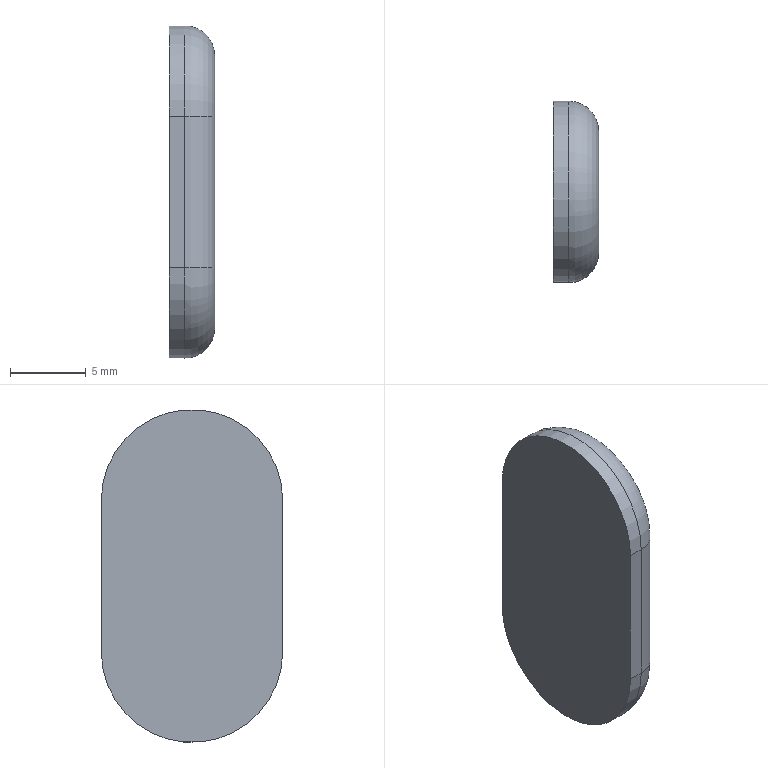Part | STEP file | 1-26.4 | 1 solid | 10 faces | box 3 x 12 x 22 mm | volume 652.172 mm3 | plane 4 | cylinder 4 | torus 2 | commonest cylinder face diameters 4 x2 12 x2
STEP:
#1=CARTESIAN_POINT('',(0.,0.,0.));
#2=DIRECTION('',(0.,0.,1.));
#3=DIRECTION('',(1.,0.,0.));
#4=AXIS2_PLACEMENT_3D('',#1,#2,#3);
#5=CARTESIAN_POINT('',(-3.,6.,5.));
#6=VERTEX_POINT('',#5);
#7=CARTESIAN_POINT('',(-3.,-6.,5.));
#8=VERTEX_POINT('',#7);
#9=CARTESIAN_POINT('',(-3.,0.,5.));
#10=DIRECTION('',(1.,0.,0.));
#11=DIRECTION('',(0.,1.,0.));
#12=AXIS2_PLACEMENT_3D('',#9,#10,#11);
#13=CIRCLE('',#12,6.);
#14=CARTESIAN_POINT('',(-3.,5.,0.));
#15=DIRECTION('',(1.,0.,0.));
#16=DIRECTION('',(0.,1.,0.));
#17=AXIS2_PLACEMENT_3D('',#14,#15,#16);
#18=PLANE('',#17);
#19=CARTESIAN_POINT('',(-5.,5.));
#20=DIRECTION('',(1.,0.));
#21=AXIS2_PLACEMENT_2D('',#19,#20);
#22=CIRCLE('',#21,6.);
#23=(GEOMETRIC_REPRESENTATION_CONTEXT(2)PARAMETRIC_REPRESENTATION_CONTEXT()REPRESENTATION_CONTEXT('',''));
#24=DEFINITIONAL_REPRESENTATION('',(#22),#23);
#25=PCURVE('',#18,#24);
#26=CARTESIAN_POINT('',(0.,0.,5.));
#27=DIRECTION('',(-1.,0.,0.));
#28=DIRECTION('',(0.,1.,0.));
#29=AXIS2_PLACEMENT_3D('',#26,#27,#28);
#30=CYLINDRICAL_SURFACE('',#29,6.);
#31=CARTESIAN_POINT('',(6.283,3.));
#32=DIRECTION('',(-1.,0.));
#33=VECTOR('',#32,1.);
#34=LINE('',#31,#33);
#35=(GEOMETRIC_REPRESENTATION_CONTEXT(2)PARAMETRIC_REPRESENTATION_CONTEXT()REPRESENTATION_CONTEXT('',''));
#36=DEFINITIONAL_REPRESENTATION('',(#34),#35);
#37=PCURVE('',#30,#36);
#38=SURFACE_CURVE('',#13,(#25,#37),.PCURVE_S1.);
#39=EDGE_CURVE('',#6,#8,#38,.T.);
#40=ORIENTED_EDGE('',*,*,#39,.T.);
#41=CARTESIAN_POINT('',(-3.,-6.,-5.));
#42=VERTEX_POINT('',#41);
#43=CARTESIAN_POINT('',(-3.,-6.,5.));
#44=DIRECTION('',(0.,0.,-1.));
#45=VECTOR('',#44,1.);
#46=LINE('',#43,#45);
#47=CARTESIAN_POINT('',(-11.,5.));
#48=DIRECTION('',(0.,-1.));
#49=VECTOR('',#48,1.);
#50=LINE('',#47,#49);
#51=(GEOMETRIC_REPRESENTATION_CONTEXT(2)PARAMETRIC_REPRESENTATION_CONTEXT()REPRESENTATION_CONTEXT('',''));
#52=DEFINITIONAL_REPRESENTATION('',(#50),#51);
#53=PCURVE('',#18,#52);
#54=CARTESIAN_POINT('',(-1.5,-6.,0.));
#55=DIRECTION('',(0.,1.,0.));
#56=DIRECTION('',(0.,0.,-1.));
#57=AXIS2_PLACEMENT_3D('',#54,#55,#56);
#58=PLANE('',#57);
#59=CARTESIAN_POINT('',(-5.,1.5));
#60=DIRECTION('',(1.,0.));
#61=VECTOR('',#60,1.);
#62=LINE('',#59,#61);
#63=(GEOMETRIC_REPRESENTATION_CONTEXT(2)PARAMETRIC_REPRESENTATION_CONTEXT()REPRESENTATION_CONTEXT('',''));
#64=DEFINITIONAL_REPRESENTATION('',(#62),#63);
#65=PCURVE('',#58,#64);
#66=SURFACE_CURVE('',#46,(#53,#65),.PCURVE_S1.);
#67=EDGE_CURVE('',#8,#42,#66,.T.);
#68=ORIENTED_EDGE('',*,*,#67,.T.);
#69=CARTESIAN_POINT('',(-3.,6.,-5.));
#70=VERTEX_POINT('',#69);
#71=CARTESIAN_POINT('',(-3.,0.,-5.));
#72=DIRECTION('',(1.,0.,0.));
#73=DIRECTION('',(0.,-1.,0.));
#74=AXIS2_PLACEMENT_3D('',#71,#72,#73);
#75=CIRCLE('',#74,6.);
#76=CARTESIAN_POINT('',(-5.,-5.));
#77=DIRECTION('',(-1.,0.));
#78=AXIS2_PLACEMENT_2D('',#76,#77);
#79=CIRCLE('',#78,6.);
#80=(GEOMETRIC_REPRESENTATION_CONTEXT(2)PARAMETRIC_REPRESENTATION_CONTEXT()REPRESENTATION_CONTEXT('',''));
#81=DEFINITIONAL_REPRESENTATION('',(#79),#80);
#82=PCURVE('',#18,#81);
#83=CARTESIAN_POINT('',(0.,0.,-5.));
#84=DIRECTION('',(-1.,0.,0.));
#85=DIRECTION('',(0.,-1.,0.));
#86=AXIS2_PLACEMENT_3D('',#83,#84,#85);
#87=CYLINDRICAL_SURFACE('',#86,6.);
#88=CARTESIAN_POINT('',(6.283,3.));
#89=DIRECTION('',(-1.,0.));
#90=VECTOR('',#89,1.);
#91=LINE('',#88,#90);
#92=(GEOMETRIC_REPRESENTATION_CONTEXT(2)PARAMETRIC_REPRESENTATION_CONTEXT()REPRESENTATION_CONTEXT('',''));
#93=DEFINITIONAL_REPRESENTATION('',(#91),#92);
#94=PCURVE('',#87,#93);
#95=SURFACE_CURVE('',#75,(#82,#94),.PCURVE_S1.);
#96=EDGE_CURVE('',#42,#70,#95,.T.);
#97=ORIENTED_EDGE('',*,*,#96,.T.);
#98=CARTESIAN_POINT('',(-3.,6.,-5.));
#99=DIRECTION('',(0.,0.,1.));
#100=VECTOR('',#99,1.);
#101=LINE('',#98,#100);
#102=CARTESIAN_POINT('',(1.,-5.));
#103=DIRECTION('',(0.,1.));
#104=VECTOR('',#103,1.);
#105=LINE('',#102,#104);
#106=(GEOMETRIC_REPRESENTATION_CONTEXT(2)PARAMETRIC_REPRESENTATION_CONTEXT()REPRESENTATION_CONTEXT('',''));
#107=DEFINITIONAL_REPRESENTATION('',(#105),#106);
#108=PCURVE('',#18,#107);
#109=CARTESIAN_POINT('',(-1.5,6.,0.));
#110=DIRECTION('',(0.,-1.,0.));
#111=DIRECTION('',(0.,0.,1.));
#112=AXIS2_PLACEMENT_3D('',#109,#110,#111);
#113=PLANE('',#112);
#114=CARTESIAN_POINT('',(-5.,1.5));
#115=DIRECTION('',(1.,0.));
#116=VECTOR('',#115,1.);
#117=LINE('',#114,#116);
#118=(GEOMETRIC_REPRESENTATION_CONTEXT(2)PARAMETRIC_REPRESENTATION_CONTEXT()REPRESENTATION_CONTEXT('',''));
#119=DEFINITIONAL_REPRESENTATION('',(#117),#118);
#120=PCURVE('',#113,#119);
#121=SURFACE_CURVE('',#101,(#108,#120),.PCURVE_S1.);
#122=EDGE_CURVE('',#70,#6,#121,.T.);
#123=ORIENTED_EDGE('',*,*,#122,.T.);
#124=EDGE_LOOP('',(#40,#68,#97,#123));
#125=FACE_BOUND('',#124,.F.);
#126=ADVANCED_FACE('',(#125),#18,.F.);
#127=CARTESIAN_POINT('',(0.,4.,5.));
#128=VERTEX_POINT('',#127);
#129=CARTESIAN_POINT('',(0.,-4.,5.));
#130=VERTEX_POINT('',#129);
#131=CARTESIAN_POINT('',(0.,0.,5.));
#132=DIRECTION('',(1.,0.,0.));
#133=DIRECTION('',(0.,1.,0.));
#134=AXIS2_PLACEMENT_3D('',#131,#132,#133);
#135=CIRCLE('',#134,4.);
#136=CARTESIAN_POINT('',(0.,5.,0.));
#137=DIRECTION('',(1.,0.,0.));
#138=DIRECTION('',(0.,1.,0.));
#139=AXIS2_PLACEMENT_3D('',#136,#137,#138);
#140=PLANE('',#139);
#141=CARTESIAN_POINT('',(-5.,5.));
#142=DIRECTION('',(1.,0.));
#143=AXIS2_PLACEMENT_2D('',#141,#142);
#144=CIRCLE('',#143,4.);
#145=(GEOMETRIC_REPRESENTATION_CONTEXT(2)PARAMETRIC_REPRESENTATION_CONTEXT()REPRESENTATION_CONTEXT('',''));
#146=DEFINITIONAL_REPRESENTATION('',(#144),#145);
#147=PCURVE('',#140,#146);
#148=CARTESIAN_POINT('',(-2.,0.,5.));
#149=DIRECTION('',(-1.,0.,0.));
#150=DIRECTION('',(0.,1.,0.));
#151=AXIS2_PLACEMENT_3D('',#148,#149,#150);
#152=TOROIDAL_SURFACE('',#151,4.,2.);
#153=CARTESIAN_POINT('',(6.283,4.712));
#154=DIRECTION('',(-1.,0.));
#155=VECTOR('',#154,1.);
#156=LINE('',#153,#155);
#157=(GEOMETRIC_REPRESENTATION_CONTEXT(2)PARAMETRIC_REPRESENTATION_CONTEXT()REPRESENTATION_CONTEXT('',''));
#158=DEFINITIONAL_REPRESENTATION('',(#156),#157);
#159=PCURVE('',#152,#158);
#160=SURFACE_CURVE('',#135,(#147,#159),.PCURVE_S1.);
#161=EDGE_CURVE('',#128,#130,#160,.T.);
#162=ORIENTED_EDGE('',*,*,#161,.T.);
#163=CARTESIAN_POINT('',(0.,-4.,-5.));
#164=VERTEX_POINT('',#163);
#165=CARTESIAN_POINT('',(0.,-4.,5.));
#166=DIRECTION('',(0.,0.,-1.));
#167=VECTOR('',#166,1.);
#168=LINE('',#165,#167);
#169=CARTESIAN_POINT('',(-9.,5.));
#170=DIRECTION('',(0.,-1.));
#171=VECTOR('',#170,1.);
#172=LINE('',#169,#171);
#173=(GEOMETRIC_REPRESENTATION_CONTEXT(2)PARAMETRIC_REPRESENTATION_CONTEXT()REPRESENTATION_CONTEXT('',''));
#174=DEFINITIONAL_REPRESENTATION('',(#172),#173);
#175=PCURVE('',#140,#174);
#176=CARTESIAN_POINT('',(-2.,-4.,5.));
#177=DIRECTION('',(0.,0.,-1.));
#178=DIRECTION('',(1.,0.,0.));
#179=AXIS2_PLACEMENT_3D('',#176,#177,#178);
#180=CYLINDRICAL_SURFACE('',#179,2.);
#181=CARTESIAN_POINT('',(0.,0.));
#182=DIRECTION('',(0.,1.));
#183=VECTOR('',#182,1.);
#184=LINE('',#181,#183);
#185=(GEOMETRIC_REPRESENTATION_CONTEXT(2)PARAMETRIC_REPRESENTATION_CONTEXT()REPRESENTATION_CONTEXT('',''));
#186=DEFINITIONAL_REPRESENTATION('',(#184),#185);
#187=PCURVE('',#180,#186);
#188=SURFACE_CURVE('',#168,(#175,#187),.PCURVE_S1.);
#189=EDGE_CURVE('',#130,#164,#188,.T.);
#190=ORIENTED_EDGE('',*,*,#189,.T.);
#191=CARTESIAN_POINT('',(0.,4.,-5.));
#192=VERTEX_POINT('',#191);
#193=CARTESIAN_POINT('',(0.,0.,-5.));
#194=DIRECTION('',(1.,0.,0.));
#195=DIRECTION('',(0.,-1.,0.));
#196=AXIS2_PLACEMENT_3D('',#193,#194,#195);
#197=CIRCLE('',#196,4.);
#198=CARTESIAN_POINT('',(-5.,-5.));
#199=DIRECTION('',(-1.,0.));
#200=AXIS2_PLACEMENT_2D('',#198,#199);
#201=CIRCLE('',#200,4.);
#202=(GEOMETRIC_REPRESENTATION_CONTEXT(2)PARAMETRIC_REPRESENTATION_CONTEXT()REPRESENTATION_CONTEXT('',''));
#203=DEFINITIONAL_REPRESENTATION('',(#201),#202);
#204=PCURVE('',#140,#203);
#205=CARTESIAN_POINT('',(-2.,0.,-5.));
#206=DIRECTION('',(-1.,0.,0.));
#207=DIRECTION('',(0.,-1.,0.));
#208=AXIS2_PLACEMENT_3D('',#205,#206,#207);
#209=TOROIDAL_SURFACE('',#208,4.,2.);
#210=CARTESIAN_POINT('',(6.283,4.712));
#211=DIRECTION('',(-1.,0.));
#212=VECTOR('',#211,1.);
#213=LINE('',#210,#212);
#214=(GEOMETRIC_REPRESENTATION_CONTEXT(2)PARAMETRIC_REPRESENTATION_CONTEXT()REPRESENTATION_CONTEXT('',''));
#215=DEFINITIONAL_REPRESENTATION('',(#213),#214);
#216=PCURVE('',#209,#215);
#217=SURFACE_CURVE('',#197,(#204,#216),.PCURVE_S1.);
#218=EDGE_CURVE('',#164,#192,#217,.T.);
#219=ORIENTED_EDGE('',*,*,#218,.T.);
#220=CARTESIAN_POINT('',(0.,4.,-5.));
#221=DIRECTION('',(0.,0.,1.));
#222=VECTOR('',#221,1.);
#223=LINE('',#220,#222);
#224=CARTESIAN_POINT('',(-1.,-5.));
#225=DIRECTION('',(0.,1.));
#226=VECTOR('',#225,1.);
#227=LINE('',#224,#226);
#228=(GEOMETRIC_REPRESENTATION_CONTEXT(2)PARAMETRIC_REPRESENTATION_CONTEXT()REPRESENTATION_CONTEXT('',''));
#229=DEFINITIONAL_REPRESENTATION('',(#227),#228);
#230=PCURVE('',#140,#229);
#231=CARTESIAN_POINT('',(-2.,4.,-5.));
#232=DIRECTION('',(0.,0.,1.));
#233=DIRECTION('',(1.,0.,0.));
#234=AXIS2_PLACEMENT_3D('',#231,#232,#233);
#235=CYLINDRICAL_SURFACE('',#234,2.);
#236=CARTESIAN_POINT('',(0.,0.));
#237=DIRECTION('',(0.,1.));
#238=VECTOR('',#237,1.);
#239=LINE('',#236,#238);
#240=(GEOMETRIC_REPRESENTATION_CONTEXT(2)PARAMETRIC_REPRESENTATION_CONTEXT()REPRESENTATION_CONTEXT('',''));
#241=DEFINITIONAL_REPRESENTATION('',(#239),#240);
#242=PCURVE('',#235,#241);
#243=SURFACE_CURVE('',#223,(#230,#242),.PCURVE_S1.);
#244=EDGE_CURVE('',#192,#128,#243,.T.);
#245=ORIENTED_EDGE('',*,*,#244,.T.);
#246=EDGE_LOOP('',(#162,#190,#219,#245));
#247=FACE_BOUND('',#246,.T.);
#248=ADVANCED_FACE('',(#247),#140,.T.);
#249=CARTESIAN_POINT('',(-2.,-6.,5.));
#250=VERTEX_POINT('',#249);
#251=CARTESIAN_POINT('',(-2.,-6.,5.));
#252=DIRECTION('',(-1.,0.,0.));
#253=VECTOR('',#252,1.);
#254=LINE('',#251,#253);
#255=CARTESIAN_POINT('',(3.142,2.));
#256=DIRECTION('',(0.,1.));
#257=VECTOR('',#256,1.);
#258=LINE('',#255,#257);
#259=(GEOMETRIC_REPRESENTATION_CONTEXT(2)PARAMETRIC_REPRESENTATION_CONTEXT()REPRESENTATION_CONTEXT('',''));
#260=DEFINITIONAL_REPRESENTATION('',(#258),#259);
#261=PCURVE('',#30,#260);
#262=CARTESIAN_POINT('',(-5.,0.5));
#263=DIRECTION('',(0.,1.));
#264=VECTOR('',#263,1.);
#265=LINE('',#262,#264);
#266=(GEOMETRIC_REPRESENTATION_CONTEXT(2)PARAMETRIC_REPRESENTATION_CONTEXT()REPRESENTATION_CONTEXT('',''));
#267=DEFINITIONAL_REPRESENTATION('',(#265),#266);
#268=PCURVE('',#58,#267);
#269=SURFACE_CURVE('',#254,(#261,#268),.PCURVE_S1.);
#270=EDGE_CURVE('',#250,#8,#269,.T.);
#271=ORIENTED_EDGE('',*,*,#270,.F.);
#272=CARTESIAN_POINT('',(-2.,6.,5.));
#273=VERTEX_POINT('',#272);
#274=CARTESIAN_POINT('',(-2.,0.,5.));
#275=DIRECTION('',(1.,0.,0.));
#276=DIRECTION('',(0.,1.,0.));
#277=AXIS2_PLACEMENT_3D('',#274,#275,#276);
#278=CIRCLE('',#277,6.);
#279=CARTESIAN_POINT('',(6.283,2.));
#280=DIRECTION('',(-1.,0.));
#281=VECTOR('',#280,1.);
#282=LINE('',#279,#281);
#283=(GEOMETRIC_REPRESENTATION_CONTEXT(2)PARAMETRIC_REPRESENTATION_CONTEXT()REPRESENTATION_CONTEXT('',''));
#284=DEFINITIONAL_REPRESENTATION('',(#282),#283);
#285=PCURVE('',#30,#284);
#286=CARTESIAN_POINT('',(6.283,6.283));
#287=DIRECTION('',(-1.,0.));
#288=VECTOR('',#287,1.);
#289=LINE('',#286,#288);
#290=(GEOMETRIC_REPRESENTATION_CONTEXT(2)PARAMETRIC_REPRESENTATION_CONTEXT()REPRESENTATION_CONTEXT('',''));
#291=DEFINITIONAL_REPRESENTATION('',(#289),#290);
#292=PCURVE('',#152,#291);
#293=SURFACE_CURVE('',#278,(#285,#292),.PCURVE_S1.);
#294=EDGE_CURVE('',#273,#250,#293,.T.);
#295=ORIENTED_EDGE('',*,*,#294,.F.);
#296=CARTESIAN_POINT('',(-2.,6.,5.));
#297=DIRECTION('',(-1.,0.,0.));
#298=VECTOR('',#297,1.);
#299=LINE('',#296,#298);
#300=CARTESIAN_POINT('',(6.283,2.));
#301=DIRECTION('',(0.,1.));
#302=VECTOR('',#301,1.);
#303=LINE('',#300,#302);
#304=(GEOMETRIC_REPRESENTATION_CONTEXT(2)PARAMETRIC_REPRESENTATION_CONTEXT()REPRESENTATION_CONTEXT('',''));
#305=DEFINITIONAL_REPRESENTATION('',(#303),#304);
#306=PCURVE('',#30,#305);
#307=CARTESIAN_POINT('',(5.,0.5));
#308=DIRECTION('',(0.,1.));
#309=VECTOR('',#308,1.);
#310=LINE('',#307,#309);
#311=(GEOMETRIC_REPRESENTATION_CONTEXT(2)PARAMETRIC_REPRESENTATION_CONTEXT()REPRESENTATION_CONTEXT('',''));
#312=DEFINITIONAL_REPRESENTATION('',(#310),#311);
#313=PCURVE('',#113,#312);
#314=SURFACE_CURVE('',#299,(#306,#313),.PCURVE_S1.);
#315=EDGE_CURVE('',#273,#6,#314,.T.);
#316=ORIENTED_EDGE('',*,*,#315,.T.);
#317=ORIENTED_EDGE('',*,*,#39,.T.);
#318=EDGE_LOOP('',(#271,#295,#316,#317));
#319=FACE_BOUND('',#318,.T.);
#320=ADVANCED_FACE('',(#319),#30,.T.);
#321=ORIENTED_EDGE('',*,*,#67,.F.);
#322=ORIENTED_EDGE('',*,*,#270,.F.);
#323=CARTESIAN_POINT('',(-2.,-6.,-5.));
#324=VERTEX_POINT('',#323);
#325=CARTESIAN_POINT('',(-2.,-6.,5.));
#326=DIRECTION('',(0.,0.,-1.));
#327=VECTOR('',#326,1.);
#328=LINE('',#325,#327);
#329=CARTESIAN_POINT('',(-5.,0.5));
#330=DIRECTION('',(1.,0.));
#331=VECTOR('',#330,1.);
#332=LINE('',#329,#331);
#333=(GEOMETRIC_REPRESENTATION_CONTEXT(2)PARAMETRIC_REPRESENTATION_CONTEXT()REPRESENTATION_CONTEXT('',''));
#334=DEFINITIONAL_REPRESENTATION('',(#332),#333);
#335=PCURVE('',#58,#334);
#336=CARTESIAN_POINT('',(1.571,0.));
#337=DIRECTION('',(0.,1.));
#338=VECTOR('',#337,1.);
#339=LINE('',#336,#338);
#340=(GEOMETRIC_REPRESENTATION_CONTEXT(2)PARAMETRIC_REPRESENTATION_CONTEXT()REPRESENTATION_CONTEXT('',''));
#341=DEFINITIONAL_REPRESENTATION('',(#339),#340);
#342=PCURVE('',#180,#341);
#343=SURFACE_CURVE('',#328,(#335,#342),.PCURVE_S1.);
#344=EDGE_CURVE('',#250,#324,#343,.T.);
#345=ORIENTED_EDGE('',*,*,#344,.T.);
#346=CARTESIAN_POINT('',(-2.,-6.,-5.));
#347=DIRECTION('',(-1.,0.,0.));
#348=VECTOR('',#347,1.);
#349=LINE('',#346,#348);
#350=CARTESIAN_POINT('',(5.,0.5));
#351=DIRECTION('',(0.,1.));
#352=VECTOR('',#351,1.);
#353=LINE('',#350,#352);
#354=(GEOMETRIC_REPRESENTATION_CONTEXT(2)PARAMETRIC_REPRESENTATION_CONTEXT()REPRESENTATION_CONTEXT('',''));
#355=DEFINITIONAL_REPRESENTATION('',(#353),#354);
#356=PCURVE('',#58,#355);
#357=CARTESIAN_POINT('',(6.283,2.));
#358=DIRECTION('',(0.,1.));
#359=VECTOR('',#358,1.);
#360=LINE('',#357,#359);
#361=(GEOMETRIC_REPRESENTATION_CONTEXT(2)PARAMETRIC_REPRESENTATION_CONTEXT()REPRESENTATION_CONTEXT('',''));
#362=DEFINITIONAL_REPRESENTATION('',(#360),#361);
#363=PCURVE('',#87,#362);
#364=SURFACE_CURVE('',#349,(#356,#363),.PCURVE_S1.);
#365=EDGE_CURVE('',#324,#42,#364,.T.);
#366=ORIENTED_EDGE('',*,*,#365,.T.);
#367=EDGE_LOOP('',(#321,#322,#345,#366));
#368=FACE_BOUND('',#367,.F.);
#369=ADVANCED_FACE('',(#368),#58,.F.);
#370=CARTESIAN_POINT('',(-2.,6.,-5.));
#371=VERTEX_POINT('',#370);
#372=CARTESIAN_POINT('',(-2.,6.,-5.));
#373=DIRECTION('',(-1.,0.,0.));
#374=VECTOR('',#373,1.);
#375=LINE('',#372,#374);
#376=CARTESIAN_POINT('',(3.142,2.));
#377=DIRECTION('',(0.,1.));
#378=VECTOR('',#377,1.);
#379=LINE('',#376,#378);
#380=(GEOMETRIC_REPRESENTATION_CONTEXT(2)PARAMETRIC_REPRESENTATION_CONTEXT()REPRESENTATION_CONTEXT('',''));
#381=DEFINITIONAL_REPRESENTATION('',(#379),#380);
#382=PCURVE('',#87,#381);
#383=CARTESIAN_POINT('',(-5.,0.5));
#384=DIRECTION('',(0.,1.));
#385=VECTOR('',#384,1.);
#386=LINE('',#383,#385);
#387=(GEOMETRIC_REPRESENTATION_CONTEXT(2)PARAMETRIC_REPRESENTATION_CONTEXT()REPRESENTATION_CONTEXT('',''));
#388=DEFINITIONAL_REPRESENTATION('',(#386),#387);
#389=PCURVE('',#113,#388);
#390=SURFACE_CURVE('',#375,(#382,#389),.PCURVE_S1.);
#391=EDGE_CURVE('',#371,#70,#390,.T.);
#392=ORIENTED_EDGE('',*,*,#391,.F.);
#393=CARTESIAN_POINT('',(-2.,0.,-5.));
#394=DIRECTION('',(1.,0.,0.));
#395=DIRECTION('',(0.,-1.,0.));
#396=AXIS2_PLACEMENT_3D('',#393,#394,#395);
#397=CIRCLE('',#396,6.);
#398=CARTESIAN_POINT('',(6.283,2.));
#399=DIRECTION('',(-1.,0.));
#400=VECTOR('',#399,1.);
#401=LINE('',#398,#400);
#402=(GEOMETRIC_REPRESENTATION_CONTEXT(2)PARAMETRIC_REPRESENTATION_CONTEXT()REPRESENTATION_CONTEXT('',''));
#403=DEFINITIONAL_REPRESENTATION('',(#401),#402);
#404=PCURVE('',#87,#403);
#405=CARTESIAN_POINT('',(6.283,6.283));
#406=DIRECTION('',(-1.,0.));
#407=VECTOR('',#406,1.);
#408=LINE('',#405,#407);
#409=(GEOMETRIC_REPRESENTATION_CONTEXT(2)PARAMETRIC_REPRESENTATION_CONTEXT()REPRESENTATION_CONTEXT('',''));
#410=DEFINITIONAL_REPRESENTATION('',(#408),#409);
#411=PCURVE('',#209,#410);
#412=SURFACE_CURVE('',#397,(#404,#411),.PCURVE_S1.);
#413=EDGE_CURVE('',#324,#371,#412,.T.);
#414=ORIENTED_EDGE('',*,*,#413,.F.);
#415=ORIENTED_EDGE('',*,*,#365,.T.);
#416=ORIENTED_EDGE('',*,*,#96,.T.);
#417=EDGE_LOOP('',(#392,#414,#415,#416));
#418=FACE_BOUND('',#417,.T.);
#419=ADVANCED_FACE('',(#418),#87,.T.);
#420=ORIENTED_EDGE('',*,*,#122,.F.);
#421=ORIENTED_EDGE('',*,*,#391,.F.);
#422=CARTESIAN_POINT('',(-2.,6.,-5.));
#423=DIRECTION('',(0.,0.,1.));
#424=VECTOR('',#423,1.);
#425=LINE('',#422,#424);
#426=CARTESIAN_POINT('',(-5.,0.5));
#427=DIRECTION('',(1.,0.));
#428=VECTOR('',#427,1.);
#429=LINE('',#426,#428);
#430=(GEOMETRIC_REPRESENTATION_CONTEXT(2)PARAMETRIC_REPRESENTATION_CONTEXT()REPRESENTATION_CONTEXT('',''));
#431=DEFINITIONAL_REPRESENTATION('',(#429),#430);
#432=PCURVE('',#113,#431);
#433=CARTESIAN_POINT('',(1.571,0.));
#434=DIRECTION('',(0.,1.));
#435=VECTOR('',#434,1.);
#436=LINE('',#433,#435);
#437=(GEOMETRIC_REPRESENTATION_CONTEXT(2)PARAMETRIC_REPRESENTATION_CONTEXT()REPRESENTATION_CONTEXT('',''));
#438=DEFINITIONAL_REPRESENTATION('',(#436),#437);
#439=PCURVE('',#235,#438);
#440=SURFACE_CURVE('',#425,(#432,#439),.PCURVE_S1.);
#441=EDGE_CURVE('',#371,#273,#440,.T.);
#442=ORIENTED_EDGE('',*,*,#441,.T.);
#443=ORIENTED_EDGE('',*,*,#315,.T.);
#444=EDGE_LOOP('',(#420,#421,#442,#443));
#445=FACE_BOUND('',#444,.F.);
#446=ADVANCED_FACE('',(#445),#113,.F.);
#447=CARTESIAN_POINT('',(-2.,-4.,5.));
#448=DIRECTION('',(0.,0.,-1.));
#449=DIRECTION('',(1.,0.,0.));
#450=AXIS2_PLACEMENT_3D('',#447,#448,#449);
#451=CIRCLE('',#450,2.);
#452=CARTESIAN_POINT('',(3.142,4.712));
#453=DIRECTION('',(0.,1.));
#454=VECTOR('',#453,1.);
#455=LINE('',#452,#454);
#456=(GEOMETRIC_REPRESENTATION_CONTEXT(2)PARAMETRIC_REPRESENTATION_CONTEXT()REPRESENTATION_CONTEXT('',''));
#457=DEFINITIONAL_REPRESENTATION('',(#455),#456);
#458=PCURVE('',#152,#457);
#459=CARTESIAN_POINT('',(0.,0.));
#460=DIRECTION('',(1.,0.));
#461=VECTOR('',#460,1.);
#462=LINE('',#459,#461);
#463=(GEOMETRIC_REPRESENTATION_CONTEXT(2)PARAMETRIC_REPRESENTATION_CONTEXT()REPRESENTATION_CONTEXT('',''));
#464=DEFINITIONAL_REPRESENTATION('',(#462),#463);
#465=PCURVE('',#180,#464);
#466=SURFACE_CURVE('',#451,(#458,#465),.PCURVE_S1.);
#467=EDGE_CURVE('',#130,#250,#466,.T.);
#468=ORIENTED_EDGE('',*,*,#467,.F.);
#469=ORIENTED_EDGE('',*,*,#161,.F.);
#470=CARTESIAN_POINT('',(-2.,4.,5.));
#471=DIRECTION('',(0.,0.,1.));
#472=DIRECTION('',(1.,0.,0.));
#473=AXIS2_PLACEMENT_3D('',#470,#471,#472);
#474=CIRCLE('',#473,2.);
#475=CARTESIAN_POINT('',(6.283,4.712));
#476=DIRECTION('',(0.,1.));
#477=VECTOR('',#476,1.);
#478=LINE('',#475,#477);
#479=(GEOMETRIC_REPRESENTATION_CONTEXT(2)PARAMETRIC_REPRESENTATION_CONTEXT()REPRESENTATION_CONTEXT('',''));
#480=DEFINITIONAL_REPRESENTATION('',(#478),#479);
#481=PCURVE('',#152,#480);
#482=CARTESIAN_POINT('',(0.,10.));
#483=DIRECTION('',(1.,0.));
#484=VECTOR('',#483,1.);
#485=LINE('',#482,#484);
#486=(GEOMETRIC_REPRESENTATION_CONTEXT(2)PARAMETRIC_REPRESENTATION_CONTEXT()REPRESENTATION_CONTEXT('',''));
#487=DEFINITIONAL_REPRESENTATION('',(#485),#486);
#488=PCURVE('',#235,#487);
#489=SURFACE_CURVE('',#474,(#481,#488),.PCURVE_S1.);
#490=EDGE_CURVE('',#128,#273,#489,.T.);
#491=ORIENTED_EDGE('',*,*,#490,.T.);
#492=ORIENTED_EDGE('',*,*,#294,.T.);
#493=EDGE_LOOP('',(#468,#469,#491,#492));
#494=FACE_BOUND('',#493,.T.);
#495=ADVANCED_FACE('',(#494),#152,.T.);
#496=ORIENTED_EDGE('',*,*,#467,.T.);
#497=ORIENTED_EDGE('',*,*,#344,.T.);
#498=CARTESIAN_POINT('',(-2.,-4.,-5.));
#499=DIRECTION('',(0.,0.,-1.));
#500=DIRECTION('',(1.,0.,0.));
#501=AXIS2_PLACEMENT_3D('',#498,#499,#500);
#502=CIRCLE('',#501,2.);
#503=CARTESIAN_POINT('',(0.,10.));
#504=DIRECTION('',(1.,0.));
#505=VECTOR('',#504,1.);
#506=LINE('',#503,#505);
#507=(GEOMETRIC_REPRESENTATION_CONTEXT(2)PARAMETRIC_REPRESENTATION_CONTEXT()REPRESENTATION_CONTEXT('',''));
#508=DEFINITIONAL_REPRESENTATION('',(#506),#507);
#509=PCURVE('',#180,#508);
#510=CARTESIAN_POINT('',(6.283,4.712));
#511=DIRECTION('',(0.,1.));
#512=VECTOR('',#511,1.);
#513=LINE('',#510,#512);
#514=(GEOMETRIC_REPRESENTATION_CONTEXT(2)PARAMETRIC_REPRESENTATION_CONTEXT()REPRESENTATION_CONTEXT('',''));
#515=DEFINITIONAL_REPRESENTATION('',(#513),#514);
#516=PCURVE('',#209,#515);
#517=SURFACE_CURVE('',#502,(#509,#516),.PCURVE_S1.);
#518=EDGE_CURVE('',#164,#324,#517,.T.);
#519=ORIENTED_EDGE('',*,*,#518,.F.);
#520=ORIENTED_EDGE('',*,*,#189,.F.);
#521=EDGE_LOOP('',(#496,#497,#519,#520));
#522=FACE_BOUND('',#521,.T.);
#523=ADVANCED_FACE('',(#522),#180,.T.);
#524=ORIENTED_EDGE('',*,*,#518,.T.);
#525=ORIENTED_EDGE('',*,*,#413,.T.);
#526=CARTESIAN_POINT('',(-2.,4.,-5.));
#527=DIRECTION('',(0.,0.,1.));
#528=DIRECTION('',(1.,0.,0.));
#529=AXIS2_PLACEMENT_3D('',#526,#527,#528);
#530=CIRCLE('',#529,2.);
#531=CARTESIAN_POINT('',(3.142,4.712));
#532=DIRECTION('',(0.,1.));
#533=VECTOR('',#532,1.);
#534=LINE('',#531,#533);
#535=(GEOMETRIC_REPRESENTATION_CONTEXT(2)PARAMETRIC_REPRESENTATION_CONTEXT()REPRESENTATION_CONTEXT('',''));
#536=DEFINITIONAL_REPRESENTATION('',(#534),#535);
#537=PCURVE('',#209,#536);
#538=CARTESIAN_POINT('',(0.,0.));
#539=DIRECTION('',(1.,0.));
#540=VECTOR('',#539,1.);
#541=LINE('',#538,#540);
#542=(GEOMETRIC_REPRESENTATION_CONTEXT(2)PARAMETRIC_REPRESENTATION_CONTEXT()REPRESENTATION_CONTEXT('',''));
#543=DEFINITIONAL_REPRESENTATION('',(#541),#542);
#544=PCURVE('',#235,#543);
#545=SURFACE_CURVE('',#530,(#537,#544),.PCURVE_S1.);
#546=EDGE_CURVE('',#192,#371,#545,.T.);
#547=ORIENTED_EDGE('',*,*,#546,.F.);
#548=ORIENTED_EDGE('',*,*,#218,.F.);
#549=EDGE_LOOP('',(#524,#525,#547,#548));
#550=FACE_BOUND('',#549,.T.);
#551=ADVANCED_FACE('',(#550),#209,.T.);
#552=ORIENTED_EDGE('',*,*,#546,.T.);
#553=ORIENTED_EDGE('',*,*,#441,.T.);
#554=ORIENTED_EDGE('',*,*,#490,.F.);
#555=ORIENTED_EDGE('',*,*,#244,.F.);
#556=EDGE_LOOP('',(#552,#553,#554,#555));
#557=FACE_BOUND('',#556,.T.);
#558=ADVANCED_FACE('',(#557),#235,.T.);
#559=CLOSED_SHELL('',(#126,#248,#320,#369,#419,#446,#495,#523,#551,#558));
#560=MANIFOLD_SOLID_BREP('',#559);
#561=(LENGTH_UNIT()NAMED_UNIT(*)SI_UNIT(.MILLI.,.METRE.));
#562=UNCERTAINTY_MEASURE_WITH_UNIT(LENGTH_MEASURE(0.0000001),#561,'','');
#563=(NAMED_UNIT(*)PLANE_ANGLE_UNIT()SI_UNIT($,.RADIAN.));
#564=(NAMED_UNIT(*)SI_UNIT($,.STERADIAN.)SOLID_ANGLE_UNIT());
#565=(GEOMETRIC_REPRESENTATION_CONTEXT(3)GLOBAL_UNCERTAINTY_ASSIGNED_CONTEXT((#562))GLOBAL_UNIT_ASSIGNED_CONTEXT((#561,#563,#564))REPRESENTATION_CONTEXT('',''));
#566=ADVANCED_BREP_SHAPE_REPRESENTATION('',(#4,#560),#565);